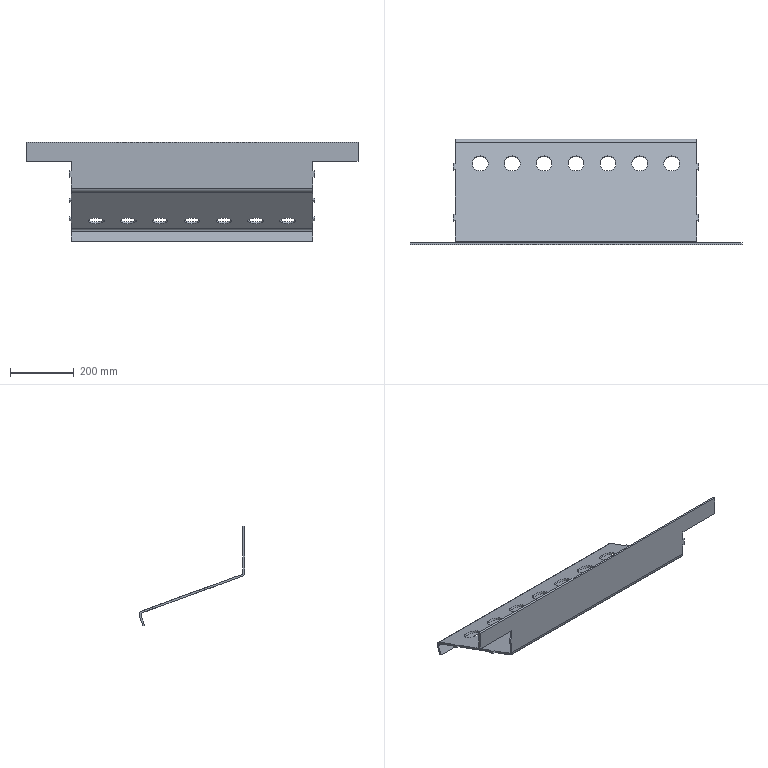Part | SolidWorks | features SMBaseFlange 3, ICE 2, FlatPattern 1, SheetMetal 1 | 1 solid | 64 faces | box 1040 x 330.948 x 311.993 mm | volume 2463441 mm3 | plane 46 | cylinder 18 | commonest cylinder face diameters 50 x14 16 x2 28 x2